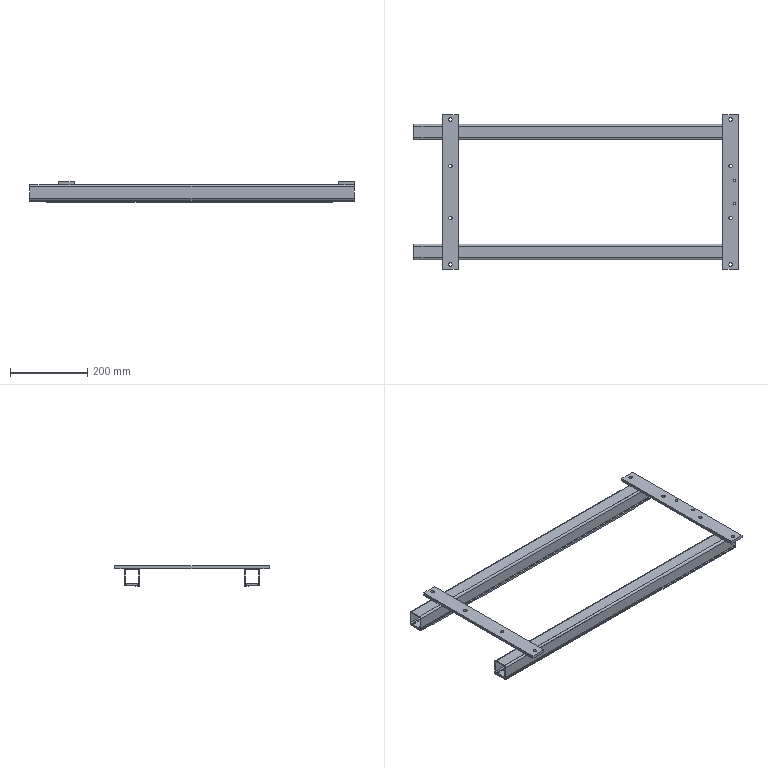Part | STEP file | 1 solid | 172 faces | box 840 x 400 x 53 mm | volume 1080937 mm3 | cylinder 120 | plane 52 | commonest cylinder face diameters 5 x92 9 x16 10 x8 7 x4